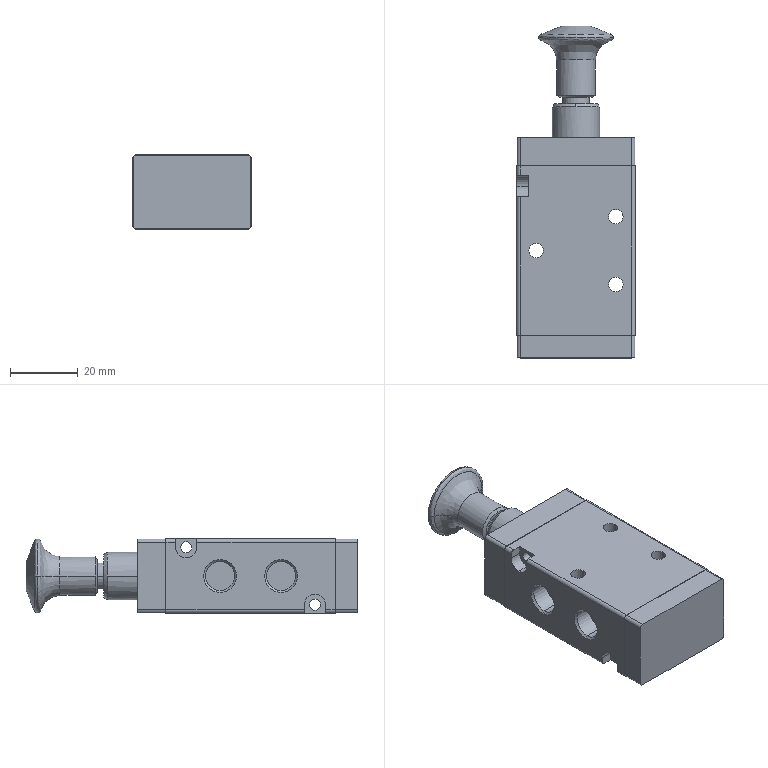Part | SolidWorks | features BaseBody 1 | 1 solid | 95 faces | box 35 x 98 x 22 mm | volume 51117 mm3 | cylinder 43 | plane 30 | cone 16 | spline 6 | commonest cylinder face diameters 2 x14 8.566 x10 4.3 x6 3.3 x4 6.3 x3 7.9 x2